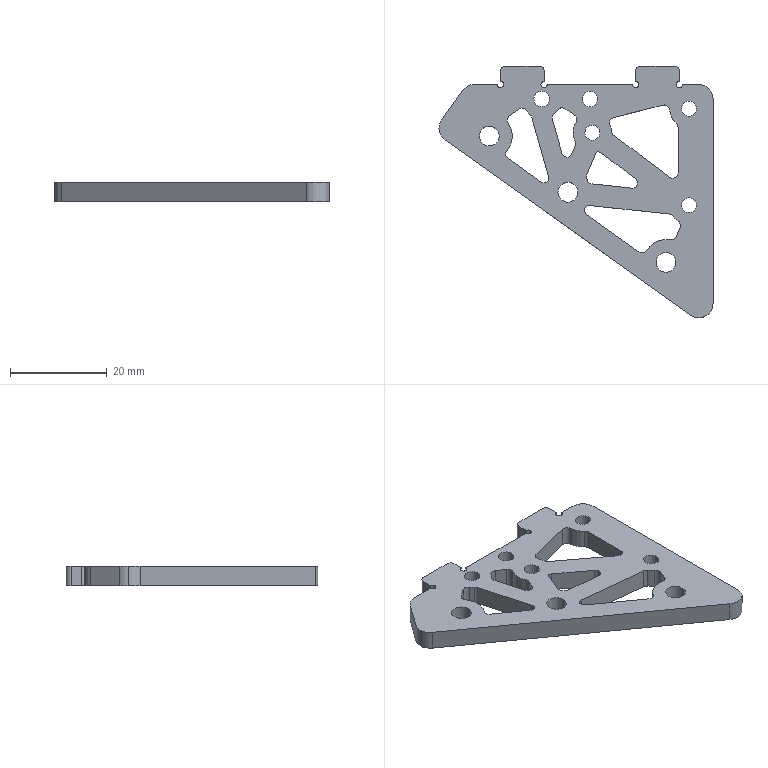Part | SolidWorks | features Fillet 3, Cut 2, ICE 2, Extrusion 1 | 1 solid | 102 faces | box 56.79 x 52.15 x 4 mm | volume 5232 mm3 | cylinder 73 | plane 29 | commonest cylinder face diameters 2.2 x32 1.3 x6 3.1 x6 4.1 x6 8 x6 6 x5